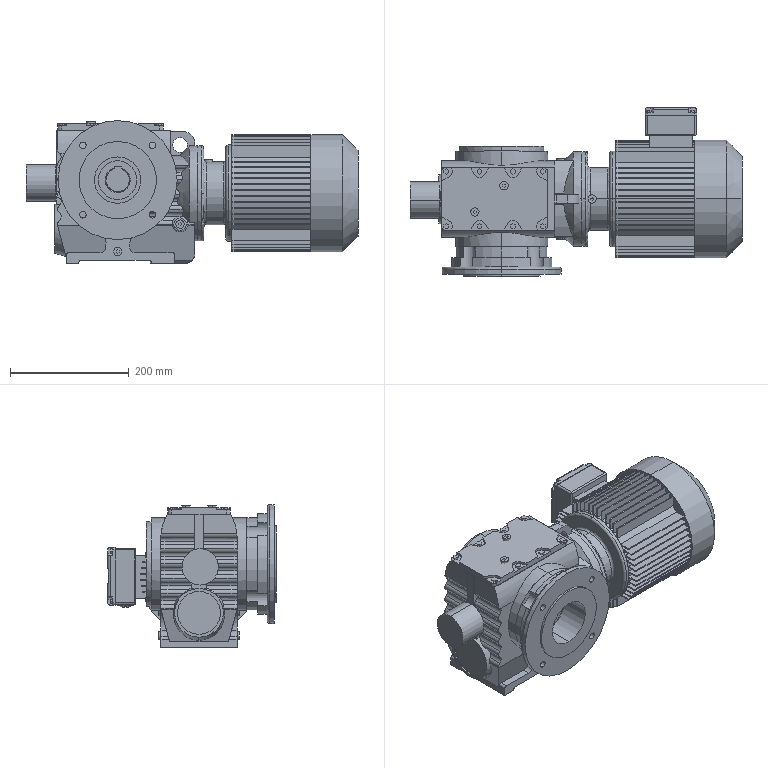Part | SolidWorks | features BaseBody 18, ICE 2 | 18 solids | 891 faces | box 558 x 283.5 x 240 mm | volume 14328030 mm3 | plane 591 | cylinder 267 | cone 17 | torus 14 | sphere 2 | commonest cylinder face diameters 15.625 x44 22.097 x44 12 x24 8 x20 20 x16 14 x14